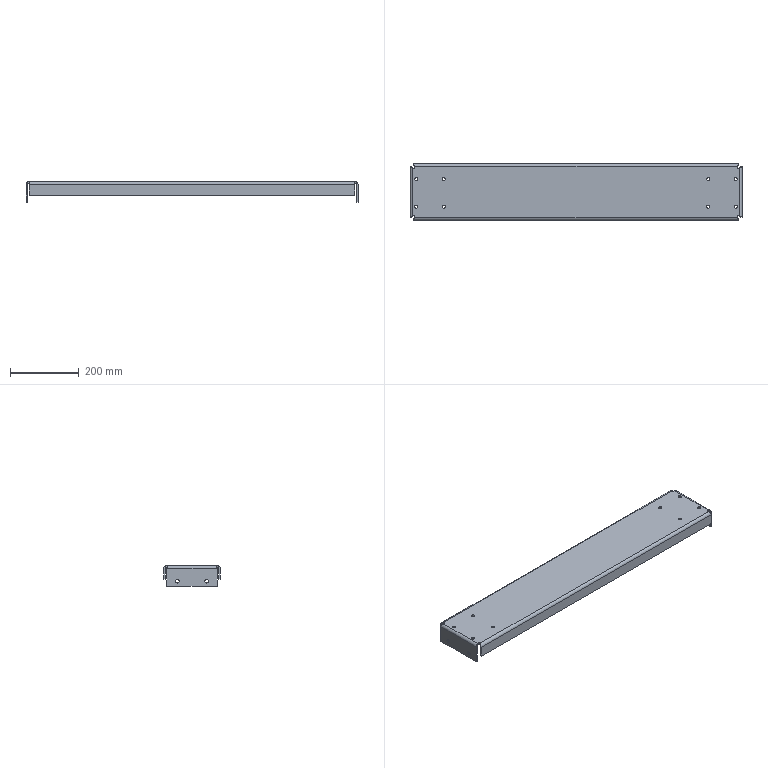Part | SolidWorks | features BaseBody 1 | 1 solid | 76 faces | box 966 x 165 x 60 mm | volume 947082 mm3 | cylinder 38 | plane 22 | spline 16 | commonest cylinder face diameters 9 x16 8 x10 11 x8 16 x4